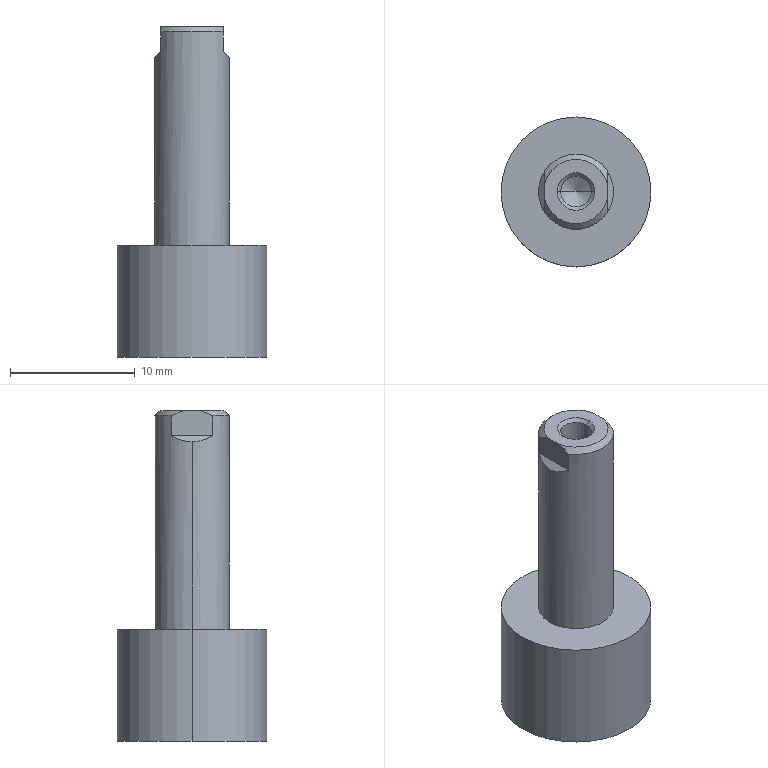Part | STEP file | HI_JSN12X10_rod_default | 1 solid | 19 faces | box 12 x 12 x 26.5 mm | volume 1467 mm3 | plane 7 | cylinder 6 | cone 6 | commonest cylinder face diameters 2.459 x2 6 x2 12 x2